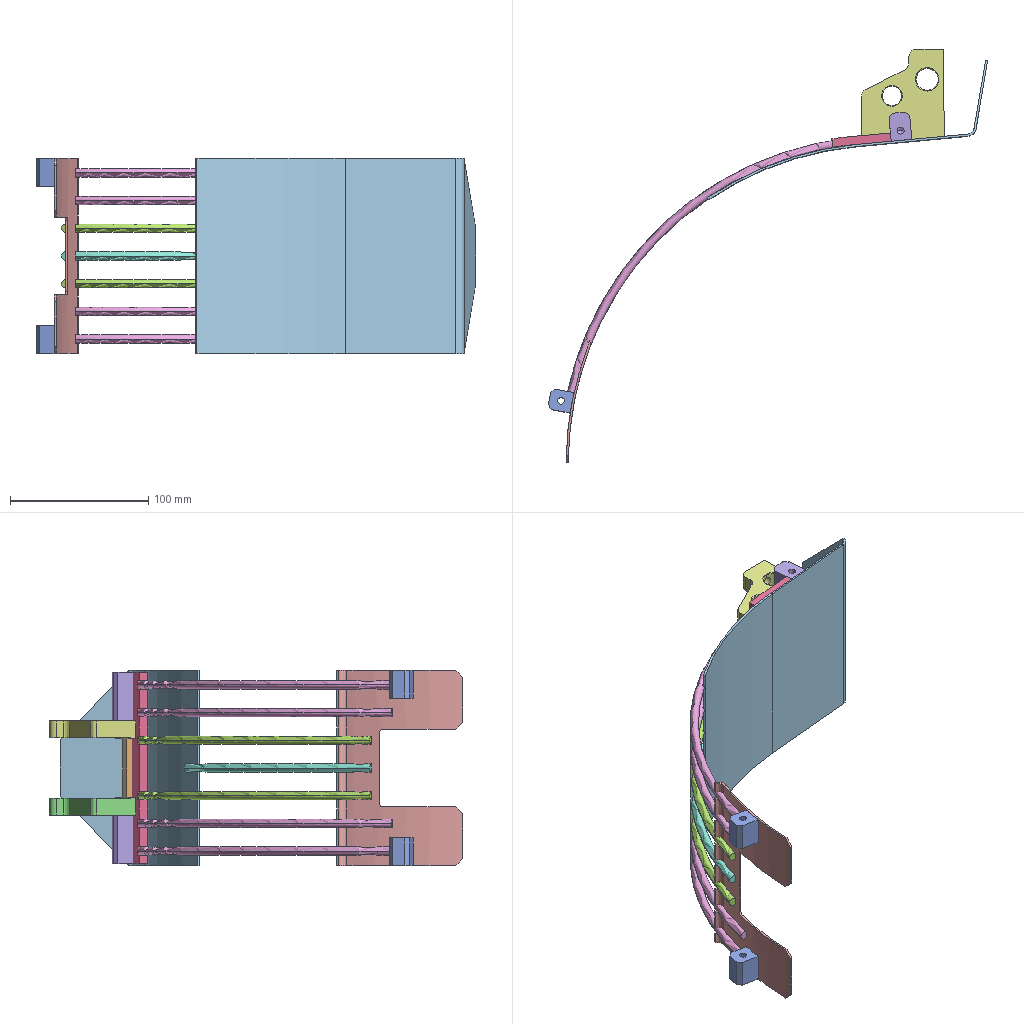Assembly | SolidWorks | 11 different items | 17 placed | box 317 x 299 x 141 mm
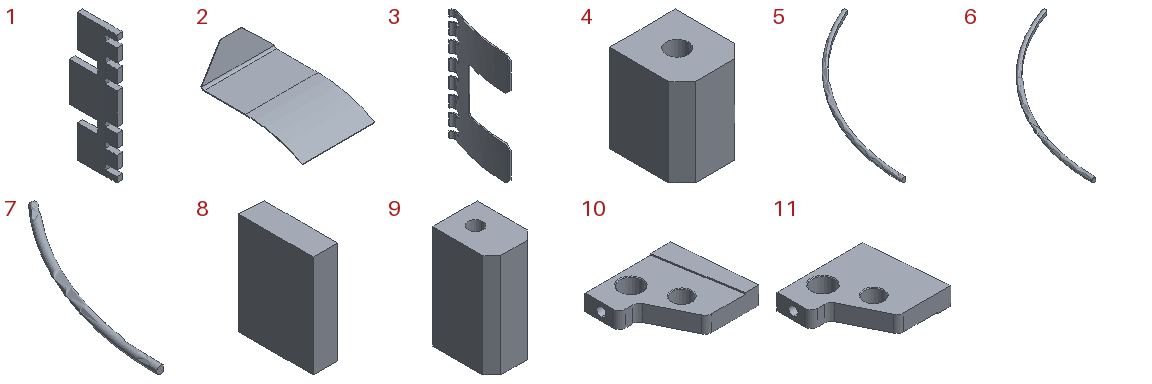Parts list (item | quantity | size | volume | features):
1 | x1 | 6.316 x 51.1 x 138 mm | 31263 mm3 | features ICE 2, Extrusion 1
2 | x1 | 141 x 210.455 x 81.673 mm | 49794 mm3 | features Chamfer 1, Extrusion 1
3 | x1 | 17.458 x 90.837 x 141 mm | 13768 mm3 | features ICE 2, Chamfer 1, Extrusion 1, Fillet 1
4 | x2 | 15 x 16.6 x 20 mm | 4383 mm3 | features Chamfer 1, Extrusion 1, HoleWzd 1
5 | x2 | 145.741 x 217.239 x 6 mm | 7317 mm3 | features ICE 1, Sweep 1
6 | x4 | 160.032 x 222.873 x 6 mm | 7707 mm3 | features ICE 1, Sweep 1
7 | x1 | 64.334 x 157.915 x 6 mm | 4754 mm3 | features ICE 1, Sweep 1
8 | x1 | 10 x 30.8 x 42 mm | 12760 mm3 | features Extrusion 1
9 | x2 | 15 x 20 x 35 mm | 9881 mm3 | features Chamfer 1, Extrusion 1, HoleWzd 1
10 | x1 | 68 x 59.543 x 13 mm | 33747 mm3 | features ICE 2, Chamfer 1, Extrusion 1
11 | x1 | 68 x 59.543 x 13 mm | 33747 mm3 | features MirrorStock 1
Mates (type | each side: item.copy, entity, surface, feature):
Symmetric | 3.1 face plane Cut-Extrude2 | 3.1 face plane Cut-Extrude2 | 5.1 plane
Symmetric | 3.1 face plane Cut-Extrude2 | 3.1 face plane Cut-Extrude2 | 7.1 plane
Coincident | 3.1 plane | assembly plane | 3 times
Symmetric | 3.1 face plane Cut-Extrude2 | 3.1 face plane Cut-Extrude2 | 6.1 plane
Concentric | 6.2 face cylinder Cut-Extrude1 | 2.1 face cylinder Boss-Extrude1
Coincident | 2.1 plane | assembly plane
Coincident | 1.1 face plane Boss-Extrude1 | 2.1 face plane Boss-Extrude1
Coincident | 1.1 plane | assembly plane
Coincident | 9.1 face plane Boss-Extrude1 | 2.1 face plane Boss-Extrude1
Coincident | 9.1 face plane Boss-Extrude1 | 1.1 face plane Boss-Extrude1
Coincident | 9.1 face plane Boss-Extrude1 | 1.1 face plane Cut-Extrude1
Coincident | 9.1 face plane Boss-Extrude1 | 9.2 face plane Boss-Extrude1 | 2 times
Coincident | 1.1 face plane Boss-Extrude1 | 9.2 face plane Boss-Extrude1
Parallel | 3.1 face cylinder Boss-Extrude1 | 5.2 face cylinder Cut-Extrude1
Coincident | 10.1 face plane Boss-Extrude1 | 9.2 face plane Boss-Extrude1
Coincident | 8.1 face plane Boss-Extrude1 | 1.1 face plane Boss-Extrude1
Coincident | 8.1 face plane Boss-Extrude1 | 2.1 face plane Boss-Extrude1
Concentric | 5.2 face cylinder Cut-Extrude1 | 2.1 face cylinder Boss-Extrude1
Concentric | 3.1 face cylinder Boss-Extrude1 | 5.2 face cylinder Cut-Extrude1
Concentric | 3.1 face cylinder Boss-Extrude1 | 4.1 face cylinder Boss-Extrude1
Concentric | 3.1 face cylinder Boss-Extrude1 | 4.2 face cylinder Boss-Extrude1
Coincident | 3.1 face plane Boss-Extrude1 | 4.2 face plane Boss-Extrude1
Coincident | 4.1 face plane Boss-Extrude1 | 4.2 face plane Boss-Extrude1
Coincident | 3.1 face plane Boss-Extrude1 | 4.1 face plane Boss-Extrude1
Concentric | 3.1 face cylinder Boss-Extrude1 | 7.1 face cylinder Cut-Extrude1
Coincident | 4.1 edge | 6.3 face plane Sweep1
Coincident | 3.1 edge | 6.2 face plane Cut-Extrude1
Coincident | 3.1 edge | 5.1 face plane Cut-Extrude1
Coincident | 3.1 edge | 7.1 face plane Cut-Extrude1
Coincident | 7.1 face plane Cut-Extrude1 | 2.1 face plane Boss-Extrude1
Coincident | 6.3 face plane Sweep1 | 1.1 edge
Coincident | 8.1 face plane Boss-Extrude1 | 10.1 face plane Boss-Extrude1